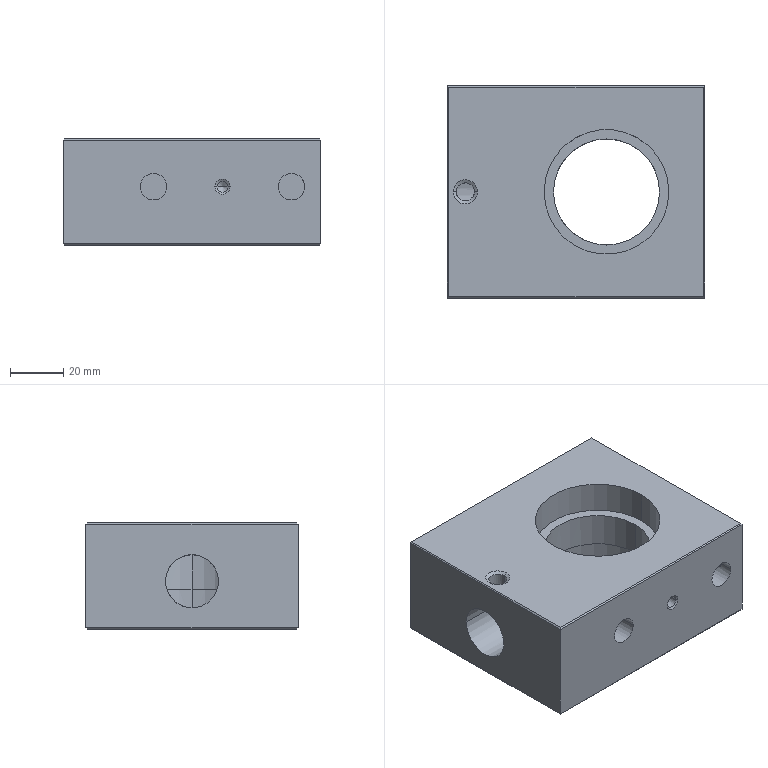Part | NX | 1 solid | 106 faces | box 97 x 80 x 40 mm | volume 227824 mm3 | cone 44 | cylinder 42 | plane 20 | commonest cylinder face diameters 4.2 x16 3.3 x8 10 x8 47 x4 6.8 x2 20 x2